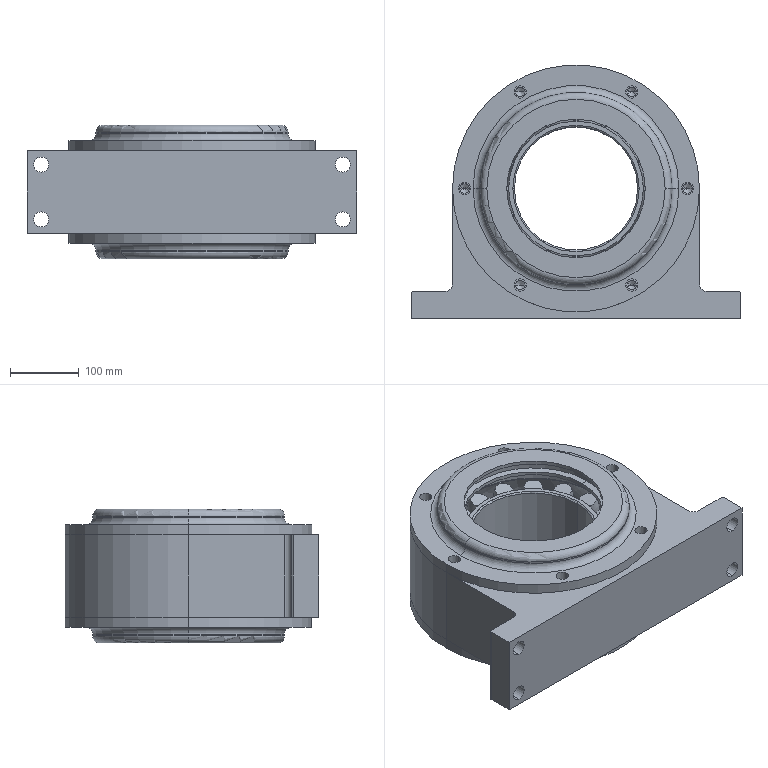Part | SolidWorks | 37 solids | 311 faces | box 480 x 370 x 194.8 mm | volume 12671030 mm3 | cylinder 101 | plane 88 | torus 88 | cone 32 | sphere 2 | commonest cylinder face diameters 14 x24 18 x24 280 x12 22 x8 202 x8 360 x5